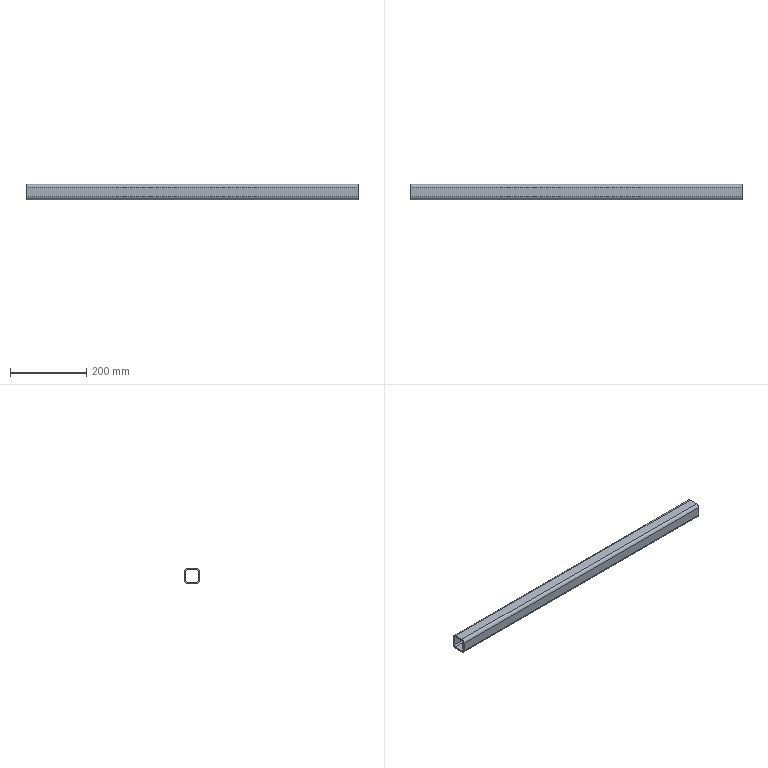Part | SolidWorks | features WeldMemberFeat 1, WeldmentFeature 1 | 1 solid | 18 faces | box 870 x 40 x 40 mm | volume 465273 mm3 | plane 10 | cylinder 8 | commonest cylinder face diameters 8 x4 16 x4
STEP:
#1=CARTESIAN_POINT('',(-1000.,20.,12.));
#2=VERTEX_POINT('',#1);
#3=CARTESIAN_POINT('',(-1000.,12.,20.));
#4=VERTEX_POINT('',#3);
#5=CARTESIAN_POINT('',(-1000.,12.,12.));
#6=DIRECTION('',(1.,0.,0.));
#7=DIRECTION('',(0.,0.,-1.));
#8=AXIS2_PLACEMENT_3D('',#5,#6,#7);
#9=CIRCLE('',#8,8.);
#10=EDGE_CURVE('',#2,#4,#9,.T.);
#11=ORIENTED_EDGE('',*,*,#10,.T.);
#12=CARTESIAN_POINT('',(-130.,12.,20.));
#13=VERTEX_POINT('',#12);
#14=CARTESIAN_POINT('',(-130.,12.,20.));
#15=DIRECTION('',(-1.,0.,0.));
#16=VECTOR('',#15,1000.);
#17=LINE('',#14,#16);
#18=EDGE_CURVE('',#13,#4,#17,.T.);
#19=ORIENTED_EDGE('',*,*,#18,.F.);
#20=CARTESIAN_POINT('',(-130.,20.,12.));
#21=VERTEX_POINT('',#20);
#22=CARTESIAN_POINT('',(-130.,12.,12.));
#23=DIRECTION('',(1.,0.,0.));
#24=DIRECTION('',(0.,0.,-1.));
#25=AXIS2_PLACEMENT_3D('',#22,#23,#24);
#26=CIRCLE('',#25,8.);
#27=EDGE_CURVE('',#21,#13,#26,.T.);
#28=ORIENTED_EDGE('',*,*,#27,.F.);
#29=CARTESIAN_POINT('',(-130.,20.,12.));
#30=DIRECTION('',(-1.,0.,0.));
#31=VECTOR('',#30,1000.);
#32=LINE('',#29,#31);
#33=EDGE_CURVE('',#21,#2,#32,.T.);
#34=ORIENTED_EDGE('',*,*,#33,.T.);
#35=EDGE_LOOP('',(#11,#19,#28,#34));
#36=FACE_OUTER_BOUND('',#35,.T.);
#37=CARTESIAN_POINT('',(-130.,12.,12.));
#38=DIRECTION('',(-1.,0.,0.));
#39=DIRECTION('',(0.,0.,1.));
#40=AXIS2_PLACEMENT_3D('',#37,#38,#39);
#41=CYLINDRICAL_SURFACE('',#40,8.);
#42=ADVANCED_FACE('',(#36),#41,.T.);
#43=CARTESIAN_POINT('',(-1000.,-12.,20.));
#44=VERTEX_POINT('',#43);
#45=CARTESIAN_POINT('',(-1000.,12.,20.));
#46=DIRECTION('',(0.,-1.,0.));
#47=VECTOR('',#46,1000.);
#48=LINE('',#45,#47);
#49=EDGE_CURVE('',#4,#44,#48,.T.);
#50=ORIENTED_EDGE('',*,*,#49,.T.);
#51=CARTESIAN_POINT('',(-130.,-12.,20.));
#52=VERTEX_POINT('',#51);
#53=CARTESIAN_POINT('',(-130.,-12.,20.));
#54=DIRECTION('',(-1.,0.,0.));
#55=VECTOR('',#54,1000.);
#56=LINE('',#53,#55);
#57=EDGE_CURVE('',#52,#44,#56,.T.);
#58=ORIENTED_EDGE('',*,*,#57,.F.);
#59=CARTESIAN_POINT('',(-130.,12.,20.));
#60=DIRECTION('',(0.,-1.,0.));
#61=VECTOR('',#60,1000.);
#62=LINE('',#59,#61);
#63=EDGE_CURVE('',#13,#52,#62,.T.);
#64=ORIENTED_EDGE('',*,*,#63,.F.);
#65=ORIENTED_EDGE('',*,*,#18,.T.);
#66=EDGE_LOOP('',(#50,#58,#64,#65));
#67=FACE_OUTER_BOUND('',#66,.T.);
#68=CARTESIAN_POINT('',(-130.,12.,20.));
#69=DIRECTION('',(0.,0.,-1.));
#70=DIRECTION('',(-1.,0.,0.));
#71=AXIS2_PLACEMENT_3D('',#68,#69,#70);
#72=PLANE('',#71);
#73=ADVANCED_FACE('',(#67),#72,.F.);
#74=CARTESIAN_POINT('',(-1000.,-20.,12.));
#75=VERTEX_POINT('',#74);
#76=CARTESIAN_POINT('',(-1000.,-12.,12.));
#77=DIRECTION('',(1.,0.,0.));
#78=DIRECTION('',(0.,0.,-1.));
#79=AXIS2_PLACEMENT_3D('',#76,#77,#78);
#80=CIRCLE('',#79,8.);
#81=EDGE_CURVE('',#44,#75,#80,.T.);
#82=ORIENTED_EDGE('',*,*,#81,.T.);
#83=CARTESIAN_POINT('',(-130.,-20.,12.));
#84=VERTEX_POINT('',#83);
#85=CARTESIAN_POINT('',(-130.,-20.,12.));
#86=DIRECTION('',(-1.,0.,0.));
#87=VECTOR('',#86,1000.);
#88=LINE('',#85,#87);
#89=EDGE_CURVE('',#84,#75,#88,.T.);
#90=ORIENTED_EDGE('',*,*,#89,.F.);
#91=CARTESIAN_POINT('',(-130.,-12.,12.));
#92=DIRECTION('',(1.,0.,0.));
#93=DIRECTION('',(0.,0.,-1.));
#94=AXIS2_PLACEMENT_3D('',#91,#92,#93);
#95=CIRCLE('',#94,8.);
#96=EDGE_CURVE('',#52,#84,#95,.T.);
#97=ORIENTED_EDGE('',*,*,#96,.F.);
#98=ORIENTED_EDGE('',*,*,#57,.T.);
#99=EDGE_LOOP('',(#82,#90,#97,#98));
#100=FACE_OUTER_BOUND('',#99,.T.);
#101=CARTESIAN_POINT('',(-130.,-12.,12.));
#102=DIRECTION('',(-1.,0.,0.));
#103=DIRECTION('',(0.,0.,1.));
#104=AXIS2_PLACEMENT_3D('',#101,#102,#103);
#105=CYLINDRICAL_SURFACE('',#104,8.);
#106=ADVANCED_FACE('',(#100),#105,.T.);
#107=CARTESIAN_POINT('',(-1000.,-20.,-12.));
#108=VERTEX_POINT('',#107);
#109=CARTESIAN_POINT('',(-1000.,-20.,-12.));
#110=DIRECTION('',(0.,0.,-1.));
#111=VECTOR('',#110,1000.);
#112=LINE('',#109,#111);
#113=EDGE_CURVE('',#75,#108,#112,.T.);
#114=ORIENTED_EDGE('',*,*,#113,.T.);
#115=CARTESIAN_POINT('',(-130.,-20.,-12.));
#116=VERTEX_POINT('',#115);
#117=CARTESIAN_POINT('',(-130.,-20.,-12.));
#118=DIRECTION('',(-1.,0.,0.));
#119=VECTOR('',#118,1000.);
#120=LINE('',#117,#119);
#121=EDGE_CURVE('',#116,#108,#120,.T.);
#122=ORIENTED_EDGE('',*,*,#121,.F.);
#123=CARTESIAN_POINT('',(-130.,-20.,-12.));
#124=DIRECTION('',(0.,0.,-1.));
#125=VECTOR('',#124,1000.);
#126=LINE('',#123,#125);
#127=EDGE_CURVE('',#84,#116,#126,.T.);
#128=ORIENTED_EDGE('',*,*,#127,.F.);
#129=ORIENTED_EDGE('',*,*,#89,.T.);
#130=EDGE_LOOP('',(#114,#122,#128,#129));
#131=FACE_OUTER_BOUND('',#130,.T.);
#132=CARTESIAN_POINT('',(-130.,-20.,-12.));
#133=DIRECTION('',(0.,1.,0.));
#134=DIRECTION('',(0.,0.,1.));
#135=AXIS2_PLACEMENT_3D('',#132,#133,#134);
#136=PLANE('',#135);
#137=ADVANCED_FACE('',(#131),#136,.F.);
#138=CARTESIAN_POINT('',(-1000.,-12.,-20.));
#139=VERTEX_POINT('',#138);
#140=CARTESIAN_POINT('',(-1000.,-12.,-12.));
#141=DIRECTION('',(1.,0.,0.));
#142=DIRECTION('',(0.,0.,-1.));
#143=AXIS2_PLACEMENT_3D('',#140,#141,#142);
#144=CIRCLE('',#143,8.);
#145=EDGE_CURVE('',#108,#139,#144,.T.);
#146=ORIENTED_EDGE('',*,*,#145,.T.);
#147=CARTESIAN_POINT('',(-130.,-12.,-20.));
#148=VERTEX_POINT('',#147);
#149=CARTESIAN_POINT('',(-130.,-12.,-20.));
#150=DIRECTION('',(-1.,0.,0.));
#151=VECTOR('',#150,1000.);
#152=LINE('',#149,#151);
#153=EDGE_CURVE('',#148,#139,#152,.T.);
#154=ORIENTED_EDGE('',*,*,#153,.F.);
#155=CARTESIAN_POINT('',(-130.,-12.,-12.));
#156=DIRECTION('',(1.,0.,0.));
#157=DIRECTION('',(0.,0.,-1.));
#158=AXIS2_PLACEMENT_3D('',#155,#156,#157);
#159=CIRCLE('',#158,8.);
#160=EDGE_CURVE('',#116,#148,#159,.T.);
#161=ORIENTED_EDGE('',*,*,#160,.F.);
#162=ORIENTED_EDGE('',*,*,#121,.T.);
#163=EDGE_LOOP('',(#146,#154,#161,#162));
#164=FACE_OUTER_BOUND('',#163,.T.);
#165=CARTESIAN_POINT('',(-130.,-12.,-12.));
#166=DIRECTION('',(-1.,0.,0.));
#167=DIRECTION('',(0.,0.,1.));
#168=AXIS2_PLACEMENT_3D('',#165,#166,#167);
#169=CYLINDRICAL_SURFACE('',#168,8.);
#170=ADVANCED_FACE('',(#164),#169,.T.);
#171=CARTESIAN_POINT('',(-1000.,12.,-20.));
#172=VERTEX_POINT('',#171);
#173=CARTESIAN_POINT('',(-1000.,-12.,-20.));
#174=DIRECTION('',(0.,1.,0.));
#175=VECTOR('',#174,1000.);
#176=LINE('',#173,#175);
#177=EDGE_CURVE('',#139,#172,#176,.T.);
#178=ORIENTED_EDGE('',*,*,#177,.T.);
#179=CARTESIAN_POINT('',(-130.,12.,-20.));
#180=VERTEX_POINT('',#179);
#181=CARTESIAN_POINT('',(-130.,12.,-20.));
#182=DIRECTION('',(-1.,0.,0.));
#183=VECTOR('',#182,1000.);
#184=LINE('',#181,#183);
#185=EDGE_CURVE('',#180,#172,#184,.T.);
#186=ORIENTED_EDGE('',*,*,#185,.F.);
#187=CARTESIAN_POINT('',(-130.,-12.,-20.));
#188=DIRECTION('',(0.,1.,0.));
#189=VECTOR('',#188,1000.);
#190=LINE('',#187,#189);
#191=EDGE_CURVE('',#148,#180,#190,.T.);
#192=ORIENTED_EDGE('',*,*,#191,.F.);
#193=ORIENTED_EDGE('',*,*,#153,.T.);
#194=EDGE_LOOP('',(#178,#186,#192,#193));
#195=FACE_OUTER_BOUND('',#194,.T.);
#196=CARTESIAN_POINT('',(-130.,-12.,-20.));
#197=DIRECTION('',(0.,0.,1.));
#198=DIRECTION('',(1.,0.,0.));
#199=AXIS2_PLACEMENT_3D('',#196,#197,#198);
#200=PLANE('',#199);
#201=ADVANCED_FACE('',(#195),#200,.F.);
#202=CARTESIAN_POINT('',(-1000.,20.,-12.));
#203=VERTEX_POINT('',#202);
#204=CARTESIAN_POINT('',(-1000.,12.,-12.));
#205=DIRECTION('',(1.,0.,0.));
#206=DIRECTION('',(0.,0.,-1.));
#207=AXIS2_PLACEMENT_3D('',#204,#205,#206);
#208=CIRCLE('',#207,8.);
#209=EDGE_CURVE('',#172,#203,#208,.T.);
#210=ORIENTED_EDGE('',*,*,#209,.T.);
#211=CARTESIAN_POINT('',(-130.,20.,-12.));
#212=VERTEX_POINT('',#211);
#213=CARTESIAN_POINT('',(-130.,20.,-12.));
#214=DIRECTION('',(-1.,0.,0.));
#215=VECTOR('',#214,1000.);
#216=LINE('',#213,#215);
#217=EDGE_CURVE('',#212,#203,#216,.T.);
#218=ORIENTED_EDGE('',*,*,#217,.F.);
#219=CARTESIAN_POINT('',(-130.,12.,-12.));
#220=DIRECTION('',(1.,0.,0.));
#221=DIRECTION('',(0.,0.,-1.));
#222=AXIS2_PLACEMENT_3D('',#219,#220,#221);
#223=CIRCLE('',#222,8.);
#224=EDGE_CURVE('',#180,#212,#223,.T.);
#225=ORIENTED_EDGE('',*,*,#224,.F.);
#226=ORIENTED_EDGE('',*,*,#185,.T.);
#227=EDGE_LOOP('',(#210,#218,#225,#226));
#228=FACE_OUTER_BOUND('',#227,.T.);
#229=CARTESIAN_POINT('',(-130.,12.,-12.));
#230=DIRECTION('',(-1.,0.,0.));
#231=DIRECTION('',(0.,0.,1.));
#232=AXIS2_PLACEMENT_3D('',#229,#230,#231);
#233=CYLINDRICAL_SURFACE('',#232,8.);
#234=ADVANCED_FACE('',(#228),#233,.T.);
#235=CARTESIAN_POINT('',(-1000.,-12.,16.));
#236=VERTEX_POINT('',#235);
#237=CARTESIAN_POINT('',(-1000.,-16.,12.));
#238=VERTEX_POINT('',#237);
#239=CARTESIAN_POINT('',(-1000.,-12.,12.));
#240=DIRECTION('',(1.,0.,0.));
#241=DIRECTION('',(0.,0.,-1.));
#242=AXIS2_PLACEMENT_3D('',#239,#240,#241);
#243=CIRCLE('',#242,4.);
#244=EDGE_CURVE('',#236,#238,#243,.T.);
#245=ORIENTED_EDGE('',*,*,#244,.F.);
#246=CARTESIAN_POINT('',(-130.,-12.,16.));
#247=VERTEX_POINT('',#246);
#248=CARTESIAN_POINT('',(-130.,-12.,16.));
#249=DIRECTION('',(-1.,0.,0.));
#250=VECTOR('',#249,1000.);
#251=LINE('',#248,#250);
#252=EDGE_CURVE('',#247,#236,#251,.T.);
#253=ORIENTED_EDGE('',*,*,#252,.F.);
#254=CARTESIAN_POINT('',(-130.,-16.,12.));
#255=VERTEX_POINT('',#254);
#256=CARTESIAN_POINT('',(-130.,-12.,12.));
#257=DIRECTION('',(1.,0.,0.));
#258=DIRECTION('',(0.,0.,-1.));
#259=AXIS2_PLACEMENT_3D('',#256,#257,#258);
#260=CIRCLE('',#259,4.);
#261=EDGE_CURVE('',#247,#255,#260,.T.);
#262=ORIENTED_EDGE('',*,*,#261,.T.);
#263=CARTESIAN_POINT('',(-130.,-16.,12.));
#264=DIRECTION('',(-1.,0.,0.));
#265=VECTOR('',#264,1000.);
#266=LINE('',#263,#265);
#267=EDGE_CURVE('',#255,#238,#266,.T.);
#268=ORIENTED_EDGE('',*,*,#267,.T.);
#269=EDGE_LOOP('',(#245,#253,#262,#268));
#270=FACE_OUTER_BOUND('',#269,.T.);
#271=CARTESIAN_POINT('',(-130.,-12.,12.));
#272=DIRECTION('',(-1.,0.,0.));
#273=DIRECTION('',(0.,0.,1.));
#274=AXIS2_PLACEMENT_3D('',#271,#272,#273);
#275=CYLINDRICAL_SURFACE('',#274,4.);
#276=ADVANCED_FACE('',(#270),#275,.F.);
#277=CARTESIAN_POINT('',(-1000.,12.,16.));
#278=VERTEX_POINT('',#277);
#279=CARTESIAN_POINT('',(-1000.,12.,16.));
#280=DIRECTION('',(0.,-1.,0.));
#281=VECTOR('',#280,1000.);
#282=LINE('',#279,#281);
#283=EDGE_CURVE('',#278,#236,#282,.T.);
#284=ORIENTED_EDGE('',*,*,#283,.F.);
#285=CARTESIAN_POINT('',(-130.,12.,16.));
#286=VERTEX_POINT('',#285);
#287=CARTESIAN_POINT('',(-130.,12.,16.));
#288=DIRECTION('',(-1.,0.,0.));
#289=VECTOR('',#288,1000.);
#290=LINE('',#287,#289);
#291=EDGE_CURVE('',#286,#278,#290,.T.);
#292=ORIENTED_EDGE('',*,*,#291,.F.);
#293=CARTESIAN_POINT('',(-130.,12.,16.));
#294=DIRECTION('',(0.,-1.,0.));
#295=VECTOR('',#294,1000.);
#296=LINE('',#293,#295);
#297=EDGE_CURVE('',#286,#247,#296,.T.);
#298=ORIENTED_EDGE('',*,*,#297,.T.);
#299=ORIENTED_EDGE('',*,*,#252,.T.);
#300=EDGE_LOOP('',(#284,#292,#298,#299));
#301=FACE_OUTER_BOUND('',#300,.T.);
#302=CARTESIAN_POINT('',(-130.,12.,16.));
#303=DIRECTION('',(0.,0.,-1.));
#304=DIRECTION('',(-1.,0.,0.));
#305=AXIS2_PLACEMENT_3D('',#302,#303,#304);
#306=PLANE('',#305);
#307=ADVANCED_FACE('',(#301),#306,.T.);
#308=CARTESIAN_POINT('',(-1000.,16.,12.));
#309=VERTEX_POINT('',#308);
#310=CARTESIAN_POINT('',(-1000.,12.,12.));
#311=DIRECTION('',(1.,0.,0.));
#312=DIRECTION('',(0.,0.,-1.));
#313=AXIS2_PLACEMENT_3D('',#310,#311,#312);
#314=CIRCLE('',#313,4.);
#315=EDGE_CURVE('',#309,#278,#314,.T.);
#316=ORIENTED_EDGE('',*,*,#315,.F.);
#317=CARTESIAN_POINT('',(-130.,16.,12.));
#318=VERTEX_POINT('',#317);
#319=CARTESIAN_POINT('',(-130.,16.,12.));
#320=DIRECTION('',(-1.,0.,0.));
#321=VECTOR('',#320,1000.);
#322=LINE('',#319,#321);
#323=EDGE_CURVE('',#318,#309,#322,.T.);
#324=ORIENTED_EDGE('',*,*,#323,.F.);
#325=CARTESIAN_POINT('',(-130.,12.,12.));
#326=DIRECTION('',(1.,0.,0.));
#327=DIRECTION('',(0.,0.,-1.));
#328=AXIS2_PLACEMENT_3D('',#325,#326,#327);
#329=CIRCLE('',#328,4.);
#330=EDGE_CURVE('',#318,#286,#329,.T.);
#331=ORIENTED_EDGE('',*,*,#330,.T.);
#332=ORIENTED_EDGE('',*,*,#291,.T.);
#333=EDGE_LOOP('',(#316,#324,#331,#332));
#334=FACE_OUTER_BOUND('',#333,.T.);
#335=CARTESIAN_POINT('',(-130.,12.,12.));
#336=DIRECTION('',(-1.,0.,0.));
#337=DIRECTION('',(0.,0.,1.));
#338=AXIS2_PLACEMENT_3D('',#335,#336,#337);
#339=CYLINDRICAL_SURFACE('',#338,4.);
#340=ADVANCED_FACE('',(#334),#339,.F.);
#341=CARTESIAN_POINT('',(-1000.,16.,-12.));
#342=VERTEX_POINT('',#341);
#343=CARTESIAN_POINT('',(-1000.,16.,12.));
#344=DIRECTION('',(0.,0.,1.));
#345=VECTOR('',#344,1000.);
#346=LINE('',#343,#345);
#347=EDGE_CURVE('',#342,#309,#346,.T.);
#348=ORIENTED_EDGE('',*,*,#347,.F.);
#349=CARTESIAN_POINT('',(-130.,16.,-12.));
#350=VERTEX_POINT('',#349);
#351=CARTESIAN_POINT('',(-130.,16.,-12.));
#352=DIRECTION('',(-1.,0.,0.));
#353=VECTOR('',#352,1000.);
#354=LINE('',#351,#353);
#355=EDGE_CURVE('',#350,#342,#354,.T.);
#356=ORIENTED_EDGE('',*,*,#355,.F.);
#357=CARTESIAN_POINT('',(-130.,16.,12.));
#358=DIRECTION('',(0.,0.,1.));
#359=VECTOR('',#358,1000.);
#360=LINE('',#357,#359);
#361=EDGE_CURVE('',#350,#318,#360,.T.);
#362=ORIENTED_EDGE('',*,*,#361,.T.);
#363=ORIENTED_EDGE('',*,*,#323,.T.);
#364=EDGE_LOOP('',(#348,#356,#362,#363));
#365=FACE_OUTER_BOUND('',#364,.T.);
#366=CARTESIAN_POINT('',(-130.,16.,12.));
#367=DIRECTION('',(0.,-1.,0.));
#368=DIRECTION('',(0.,0.,-1.));
#369=AXIS2_PLACEMENT_3D('',#366,#367,#368);
#370=PLANE('',#369);
#371=ADVANCED_FACE('',(#365),#370,.T.);
#372=CARTESIAN_POINT('',(-1000.,12.,-16.));
#373=VERTEX_POINT('',#372);
#374=CARTESIAN_POINT('',(-1000.,12.,-12.));
#375=DIRECTION('',(1.,0.,0.));
#376=DIRECTION('',(0.,0.,-1.));
#377=AXIS2_PLACEMENT_3D('',#374,#375,#376);
#378=CIRCLE('',#377,4.);
#379=EDGE_CURVE('',#373,#342,#378,.T.);
#380=ORIENTED_EDGE('',*,*,#379,.F.);
#381=CARTESIAN_POINT('',(-130.,12.,-16.));
#382=VERTEX_POINT('',#381);
#383=CARTESIAN_POINT('',(-130.,12.,-16.));
#384=DIRECTION('',(-1.,0.,0.));
#385=VECTOR('',#384,1000.);
#386=LINE('',#383,#385);
#387=EDGE_CURVE('',#382,#373,#386,.T.);
#388=ORIENTED_EDGE('',*,*,#387,.F.);
#389=CARTESIAN_POINT('',(-130.,12.,-12.));
#390=DIRECTION('',(1.,0.,0.));
#391=DIRECTION('',(0.,0.,-1.));
#392=AXIS2_PLACEMENT_3D('',#389,#390,#391);
#393=CIRCLE('',#392,4.);
#394=EDGE_CURVE('',#382,#350,#393,.T.);
#395=ORIENTED_EDGE('',*,*,#394,.T.);
#396=ORIENTED_EDGE('',*,*,#355,.T.);
#397=EDGE_LOOP('',(#380,#388,#395,#396));
#398=FACE_OUTER_BOUND('',#397,.T.);
#399=CARTESIAN_POINT('',(-130.,12.,-12.));
#400=DIRECTION('',(-1.,0.,0.));
#401=DIRECTION('',(0.,0.,1.));
#402=AXIS2_PLACEMENT_3D('',#399,#400,#401);
#403=CYLINDRICAL_SURFACE('',#402,4.);
#404=ADVANCED_FACE('',(#398),#403,.F.);
#405=CARTESIAN_POINT('',(-1000.,-12.,-16.));
#406=VERTEX_POINT('',#405);
#407=CARTESIAN_POINT('',(-1000.,-12.,-16.));
#408=DIRECTION('',(0.,1.,0.));
#409=VECTOR('',#408,1000.);
#410=LINE('',#407,#409);
#411=EDGE_CURVE('',#406,#373,#410,.T.);
#412=ORIENTED_EDGE('',*,*,#411,.F.);
#413=CARTESIAN_POINT('',(-130.,-12.,-16.));
#414=VERTEX_POINT('',#413);
#415=CARTESIAN_POINT('',(-130.,-12.,-16.));
#416=DIRECTION('',(-1.,0.,0.));
#417=VECTOR('',#416,1000.);
#418=LINE('',#415,#417);
#419=EDGE_CURVE('',#414,#406,#418,.T.);
#420=ORIENTED_EDGE('',*,*,#419,.F.);
#421=CARTESIAN_POINT('',(-130.,-12.,-16.));
#422=DIRECTION('',(0.,1.,0.));
#423=VECTOR('',#422,1000.);
#424=LINE('',#421,#423);
#425=EDGE_CURVE('',#414,#382,#424,.T.);
#426=ORIENTED_EDGE('',*,*,#425,.T.);
#427=ORIENTED_EDGE('',*,*,#387,.T.);
#428=EDGE_LOOP('',(#412,#420,#426,#427));
#429=FACE_OUTER_BOUND('',#428,.T.);
#430=CARTESIAN_POINT('',(-130.,-12.,-16.));
#431=DIRECTION('',(0.,0.,1.));
#432=DIRECTION('',(1.,0.,0.));
#433=AXIS2_PLACEMENT_3D('',#430,#431,#432);
#434=PLANE('',#433);
#435=ADVANCED_FACE('',(#429),#434,.T.);
#436=CARTESIAN_POINT('',(-1000.,-16.,-12.));
#437=VERTEX_POINT('',#436);
#438=CARTESIAN_POINT('',(-1000.,-12.,-12.));
#439=DIRECTION('',(1.,0.,0.));
#440=DIRECTION('',(0.,0.,-1.));
#441=AXIS2_PLACEMENT_3D('',#438,#439,#440);
#442=CIRCLE('',#441,4.);
#443=EDGE_CURVE('',#437,#406,#442,.T.);
#444=ORIENTED_EDGE('',*,*,#443,.F.);
#445=CARTESIAN_POINT('',(-130.,-16.,-12.));
#446=VERTEX_POINT('',#445);
#447=CARTESIAN_POINT('',(-130.,-16.,-12.));
#448=DIRECTION('',(-1.,0.,0.));
#449=VECTOR('',#448,1000.);
#450=LINE('',#447,#449);
#451=EDGE_CURVE('',#446,#437,#450,.T.);
#452=ORIENTED_EDGE('',*,*,#451,.F.);
#453=CARTESIAN_POINT('',(-130.,-12.,-12.));
#454=DIRECTION('',(1.,0.,0.));
#455=DIRECTION('',(0.,0.,-1.));
#456=AXIS2_PLACEMENT_3D('',#453,#454,#455);
#457=CIRCLE('',#456,4.);
#458=EDGE_CURVE('',#446,#414,#457,.T.);
#459=ORIENTED_EDGE('',*,*,#458,.T.);
#460=ORIENTED_EDGE('',*,*,#419,.T.);
#461=EDGE_LOOP('',(#444,#452,#459,#460));
#462=FACE_OUTER_BOUND('',#461,.T.);
#463=CARTESIAN_POINT('',(-130.,-12.,-12.));
#464=DIRECTION('',(-1.,0.,0.));
#465=DIRECTION('',(0.,0.,1.));
#466=AXIS2_PLACEMENT_3D('',#463,#464,#465);
#467=CYLINDRICAL_SURFACE('',#466,4.);
#468=ADVANCED_FACE('',(#462),#467,.F.);
#469=CARTESIAN_POINT('',(-1000.,-16.,-12.));
#470=DIRECTION('',(0.,0.,-1.));
#471=VECTOR('',#470,1000.);
#472=LINE('',#469,#471);
#473=EDGE_CURVE('',#238,#437,#472,.T.);
#474=ORIENTED_EDGE('',*,*,#473,.F.);
#475=ORIENTED_EDGE('',*,*,#267,.F.);
#476=CARTESIAN_POINT('',(-130.,-16.,-12.));
#477=DIRECTION('',(0.,0.,-1.));
#478=VECTOR('',#477,1000.);
#479=LINE('',#476,#478);
#480=EDGE_CURVE('',#255,#446,#479,.T.);
#481=ORIENTED_EDGE('',*,*,#480,.T.);
#482=ORIENTED_EDGE('',*,*,#451,.T.);
#483=EDGE_LOOP('',(#474,#475,#481,#482));
#484=FACE_OUTER_BOUND('',#483,.T.);
#485=CARTESIAN_POINT('',(-130.,-16.,-12.));
#486=DIRECTION('',(0.,1.,0.));
#487=DIRECTION('',(0.,0.,1.));
#488=AXIS2_PLACEMENT_3D('',#485,#486,#487);
#489=PLANE('',#488);
#490=ADVANCED_FACE('',(#484),#489,.T.);
#491=CARTESIAN_POINT('',(-1000.,20.,12.));
#492=DIRECTION('',(0.,0.,1.));
#493=VECTOR('',#492,1000.);
#494=LINE('',#491,#493);
#495=EDGE_CURVE('',#203,#2,#494,.T.);
#496=ORIENTED_EDGE('',*,*,#495,.T.);
#497=ORIENTED_EDGE('',*,*,#33,.F.);
#498=CARTESIAN_POINT('',(-130.,20.,12.));
#499=DIRECTION('',(0.,0.,1.));
#500=VECTOR('',#499,1000.);
#501=LINE('',#498,#500);
#502=EDGE_CURVE('',#212,#21,#501,.T.);
#503=ORIENTED_EDGE('',*,*,#502,.F.);
#504=ORIENTED_EDGE('',*,*,#217,.T.);
#505=EDGE_LOOP('',(#496,#497,#503,#504));
#506=FACE_OUTER_BOUND('',#505,.T.);
#507=CARTESIAN_POINT('',(-130.,20.,12.));
#508=DIRECTION('',(0.,-1.,0.));
#509=DIRECTION('',(0.,0.,-1.));
#510=AXIS2_PLACEMENT_3D('',#507,#508,#509);
#511=PLANE('',#510);
#512=ADVANCED_FACE('',(#506),#511,.F.);
#513=ORIENTED_EDGE('',*,*,#261,.F.);
#514=ORIENTED_EDGE('',*,*,#297,.F.);
#515=ORIENTED_EDGE('',*,*,#330,.F.);
#516=ORIENTED_EDGE('',*,*,#361,.F.);
#517=ORIENTED_EDGE('',*,*,#394,.F.);
#518=ORIENTED_EDGE('',*,*,#425,.F.);
#519=ORIENTED_EDGE('',*,*,#458,.F.);
#520=ORIENTED_EDGE('',*,*,#480,.F.);
#521=EDGE_LOOP('',(#513,#514,#515,#516,#517,#518,#519,#520));
#522=FACE_BOUND('',#521,.T.);
#523=ORIENTED_EDGE('',*,*,#27,.T.);
#524=ORIENTED_EDGE('',*,*,#63,.T.);
#525=ORIENTED_EDGE('',*,*,#96,.T.);
#526=ORIENTED_EDGE('',*,*,#127,.T.);
#527=ORIENTED_EDGE('',*,*,#160,.T.);
#528=ORIENTED_EDGE('',*,*,#191,.T.);
#529=ORIENTED_EDGE('',*,*,#224,.T.);
#530=ORIENTED_EDGE('',*,*,#502,.T.);
#531=EDGE_LOOP('',(#523,#524,#525,#526,#527,#528,#529,#530));
#532=FACE_OUTER_BOUND('',#531,.T.);
#533=CARTESIAN_POINT('',(-130.,12.,12.));
#534=DIRECTION('',(1.,0.,0.));
#535=DIRECTION('',(0.,0.,-1.));
#536=AXIS2_PLACEMENT_3D('',#533,#534,#535);
#537=PLANE('',#536);
#538=ADVANCED_FACE('',(#522,#532),#537,.T.);
#539=ORIENTED_EDGE('',*,*,#244,.T.);
#540=ORIENTED_EDGE('',*,*,#473,.T.);
#541=ORIENTED_EDGE('',*,*,#443,.T.);
#542=ORIENTED_EDGE('',*,*,#411,.T.);
#543=ORIENTED_EDGE('',*,*,#379,.T.);
#544=ORIENTED_EDGE('',*,*,#347,.T.);
#545=ORIENTED_EDGE('',*,*,#315,.T.);
#546=ORIENTED_EDGE('',*,*,#283,.T.);
#547=EDGE_LOOP('',(#539,#540,#541,#542,#543,#544,#545,#546));
#548=FACE_BOUND('',#547,.T.);
#549=ORIENTED_EDGE('',*,*,#10,.F.);
#550=ORIENTED_EDGE('',*,*,#495,.F.);
#551=ORIENTED_EDGE('',*,*,#209,.F.);
#552=ORIENTED_EDGE('',*,*,#177,.F.);
#553=ORIENTED_EDGE('',*,*,#145,.F.);
#554=ORIENTED_EDGE('',*,*,#113,.F.);
#555=ORIENTED_EDGE('',*,*,#81,.F.);
#556=ORIENTED_EDGE('',*,*,#49,.F.);
#557=EDGE_LOOP('',(#549,#550,#551,#552,#553,#554,#555,#556));
#558=FACE_OUTER_BOUND('',#557,.T.);
#559=CARTESIAN_POINT('',(-1000.,12.,12.));
#560=DIRECTION('',(1.,0.,0.));
#561=DIRECTION('',(0.,0.,-1.));
#562=AXIS2_PLACEMENT_3D('',#559,#560,#561);
#563=PLANE('',#562);
#564=ADVANCED_FACE('',(#548,#558),#563,.F.);
#565=CLOSED_SHELL('',(#42,#73,#106,#137,#170,#201,#234,#276,#307,#340,#371,#404,#435,#468,#490,#512,#538,#564));
#566=MANIFOLD_SOLID_BREP('',#565);
#567=CARTESIAN_POINT('',(0.,0.,0.));
#568=DIRECTION('',(0.,0.,1.));
#569=DIRECTION('',(1.,0.,0.));
#570=AXIS2_PLACEMENT_3D('',#567,#568,#569);
#571=(LENGTH_UNIT()NAMED_UNIT(*)SI_UNIT(.MILLI.,.METRE.));
#572=UNCERTAINTY_MEASURE_WITH_UNIT(LENGTH_MEASURE(0.00001),#571,'','');
#573=(NAMED_UNIT(*)PLANE_ANGLE_UNIT()SI_UNIT($,.RADIAN.));
#574=(NAMED_UNIT(*)SI_UNIT($,.STERADIAN.)SOLID_ANGLE_UNIT());
#575=(GEOMETRIC_REPRESENTATION_CONTEXT(3)GLOBAL_UNCERTAINTY_ASSIGNED_CONTEXT((#572))GLOBAL_UNIT_ASSIGNED_CONTEXT((#571,#573,#574))REPRESENTATION_CONTEXT('',''));
#576=ADVANCED_BREP_SHAPE_REPRESENTATION('',(#566,#570),#575);